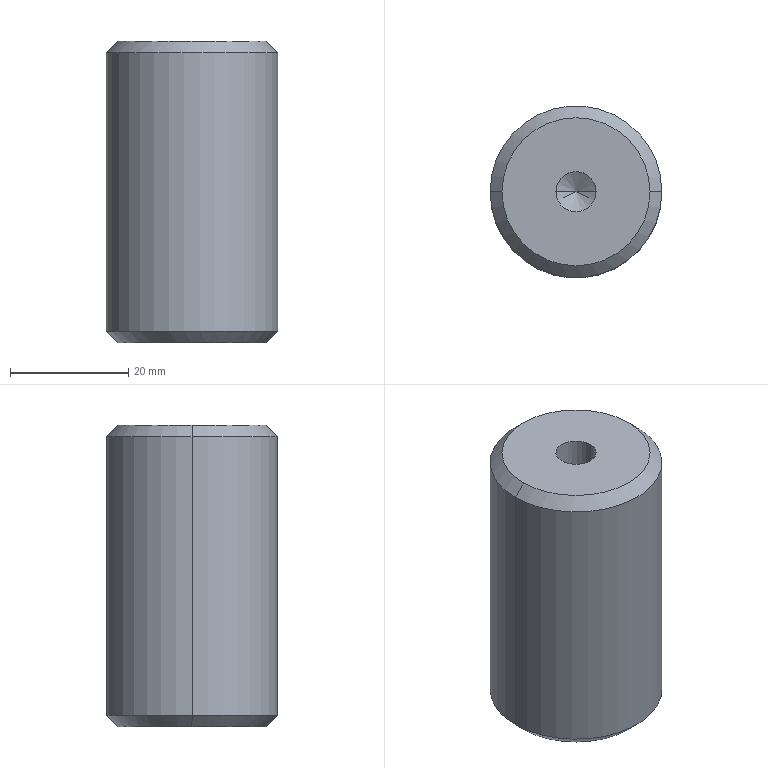Part | STEP file | BU-A03b#180 | 1 solid | 16 faces | box 29 x 29 x 51 mm | volume 31619 mm3 | cone 8 | cylinder 6 | plane 2 | commonest cylinder face diameters 6.8 x4 29 x2
STEP:
#1=CARTESIAN_POINT('',(0.,0.,0.));
#2=DIRECTION('',(0.,0.,1.));
#3=DIRECTION('',(1.,0.,0.));
#4=AXIS2_PLACEMENT_3D('',#1,#2,#3);
#5=CARTESIAN_POINT('',(12.5,0.,51.));
#6=VERTEX_POINT('',#5);
#7=CARTESIAN_POINT('',(-12.5,0.,51.));
#8=VERTEX_POINT('',#7);
#9=CARTESIAN_POINT('',(0.,0.,51.));
#10=DIRECTION('',(0.,0.,1.));
#11=DIRECTION('',(1.,0.,0.));
#12=AXIS2_PLACEMENT_3D('',#9,#10,#11);
#13=CIRCLE('',#12,12.5);
#14=CARTESIAN_POINT('',(0.,0.,51.));
#15=DIRECTION('',(0.,0.,-1.));
#16=DIRECTION('',(-1.,0.,0.));
#17=AXIS2_PLACEMENT_3D('',#14,#15,#16);
#18=CONICAL_SURFACE('',#17,12.5,0.7854);
#19=CARTESIAN_POINT('',(3.142,0.));
#20=DIRECTION('',(-1.,0.));
#21=VECTOR('',#20,1.);
#22=LINE('',#19,#21);
#23=(GEOMETRIC_REPRESENTATION_CONTEXT(2)PARAMETRIC_REPRESENTATION_CONTEXT()REPRESENTATION_CONTEXT('',''));
#24=DEFINITIONAL_REPRESENTATION('',(#22),#23);
#25=PCURVE('',#18,#24);
#26=CARTESIAN_POINT('',(0.,0.,51.));
#27=DIRECTION('',(0.,0.,1.));
#28=DIRECTION('',(1.,0.,0.));
#29=AXIS2_PLACEMENT_3D('',#26,#27,#28);
#30=PLANE('',#29);
#31=CARTESIAN_POINT('',(0.,0.));
#32=DIRECTION('',(1.,0.));
#33=AXIS2_PLACEMENT_2D('',#31,#32);
#34=CIRCLE('',#33,12.5);
#35=(GEOMETRIC_REPRESENTATION_CONTEXT(2)PARAMETRIC_REPRESENTATION_CONTEXT()REPRESENTATION_CONTEXT('',''));
#36=DEFINITIONAL_REPRESENTATION('',(#34),#35);
#37=PCURVE('',#30,#36);
#38=SURFACE_CURVE('',#13,(#25,#37),.PCURVE_S1.);
#39=EDGE_CURVE('',#6,#8,#38,.T.);
#40=ORIENTED_EDGE('',*,*,#39,.F.);
#41=CARTESIAN_POINT('',(14.5,0.,49.));
#42=VERTEX_POINT('',#41);
#43=CARTESIAN_POINT('',(12.5,0.,51.));
#44=DIRECTION('',(0.7071,0.,-0.7071));
#45=VECTOR('',#44,1.);
#46=LINE('',#43,#45);
#47=CARTESIAN_POINT('',(3.142,0.));
#48=DIRECTION('',(0.,1.));
#49=VECTOR('',#48,1.);
#50=LINE('',#47,#49);
#51=(GEOMETRIC_REPRESENTATION_CONTEXT(2)PARAMETRIC_REPRESENTATION_CONTEXT()REPRESENTATION_CONTEXT('',''));
#52=DEFINITIONAL_REPRESENTATION('',(#50),#51);
#53=PCURVE('',#18,#52);
#54=CARTESIAN_POINT('',(0.,0.,51.));
#55=DIRECTION('',(0.,0.,-1.));
#56=DIRECTION('',(-1.,0.,0.));
#57=AXIS2_PLACEMENT_3D('',#54,#55,#56);
#58=CONICAL_SURFACE('',#57,12.5,0.7854);
#59=CARTESIAN_POINT('',(3.142,0.));
#60=DIRECTION('',(0.,1.));
#61=VECTOR('',#60,1.);
#62=LINE('',#59,#61);
#63=(GEOMETRIC_REPRESENTATION_CONTEXT(2)PARAMETRIC_REPRESENTATION_CONTEXT()REPRESENTATION_CONTEXT('',''));
#64=DEFINITIONAL_REPRESENTATION('',(#62),#63);
#65=PCURVE('',#58,#64);
#66=SURFACE_CURVE('',#46,(#53,#65),.PCURVE_S1.);
#67=EDGE_CURVE('',#6,#42,#66,.T.);
#68=ORIENTED_EDGE('',*,*,#67,.T.);
#69=CARTESIAN_POINT('',(-14.5,0.,49.));
#70=VERTEX_POINT('',#69);
#71=CARTESIAN_POINT('',(0.,0.,49.));
#72=DIRECTION('',(0.,0.,-1.));
#73=DIRECTION('',(1.,0.,0.));
#74=AXIS2_PLACEMENT_3D('',#71,#72,#73);
#75=CIRCLE('',#74,14.5);
#76=CARTESIAN_POINT('',(-3.142,2.));
#77=DIRECTION('',(1.,0.));
#78=VECTOR('',#77,1.);
#79=LINE('',#76,#78);
#80=(GEOMETRIC_REPRESENTATION_CONTEXT(2)PARAMETRIC_REPRESENTATION_CONTEXT()REPRESENTATION_CONTEXT('',''));
#81=DEFINITIONAL_REPRESENTATION('',(#79),#80);
#82=PCURVE('',#18,#81);
#83=CARTESIAN_POINT('',(0.,0.,51.));
#84=DIRECTION('',(0.,0.,-1.));
#85=DIRECTION('',(-1.,0.,0.));
#86=AXIS2_PLACEMENT_3D('',#83,#84,#85);
#87=CYLINDRICAL_SURFACE('',#86,14.5);
#88=CARTESIAN_POINT('',(-3.142,2.));
#89=DIRECTION('',(1.,0.));
#90=VECTOR('',#89,1.);
#91=LINE('',#88,#90);
#92=(GEOMETRIC_REPRESENTATION_CONTEXT(2)PARAMETRIC_REPRESENTATION_CONTEXT()REPRESENTATION_CONTEXT('',''));
#93=DEFINITIONAL_REPRESENTATION('',(#91),#92);
#94=PCURVE('',#87,#93);
#95=SURFACE_CURVE('',#75,(#82,#94),.PCURVE_S1.);
#96=EDGE_CURVE('',#70,#42,#95,.T.);
#97=ORIENTED_EDGE('',*,*,#96,.F.);
#98=CARTESIAN_POINT('',(-12.5,0.,51.));
#99=DIRECTION('',(-0.7071,0.,-0.7071));
#100=VECTOR('',#99,1.);
#101=LINE('',#98,#100);
#102=CARTESIAN_POINT('',(0.,0.));
#103=DIRECTION('',(0.,1.));
#104=VECTOR('',#103,1.);
#105=LINE('',#102,#104);
#106=(GEOMETRIC_REPRESENTATION_CONTEXT(2)PARAMETRIC_REPRESENTATION_CONTEXT()REPRESENTATION_CONTEXT('',''));
#107=DEFINITIONAL_REPRESENTATION('',(#105),#106);
#108=PCURVE('',#18,#107);
#109=CARTESIAN_POINT('',(6.283,0.));
#110=DIRECTION('',(0.,1.));
#111=VECTOR('',#110,1.);
#112=LINE('',#109,#111);
#113=(GEOMETRIC_REPRESENTATION_CONTEXT(2)PARAMETRIC_REPRESENTATION_CONTEXT()REPRESENTATION_CONTEXT('',''));
#114=DEFINITIONAL_REPRESENTATION('',(#112),#113);
#115=PCURVE('',#58,#114);
#116=SURFACE_CURVE('',#101,(#108,#115),.PCURVE_S1.);
#117=EDGE_CURVE('',#8,#70,#116,.T.);
#118=ORIENTED_EDGE('',*,*,#117,.F.);
#119=EDGE_LOOP('',(#40,#68,#97,#118));
#120=FACE_BOUND('',#119,.T.);
#121=ADVANCED_FACE('',(#120),#18,.T.);
#122=CARTESIAN_POINT('',(-12.5,0.,0.));
#123=VERTEX_POINT('',#122);
#124=CARTESIAN_POINT('',(12.5,0.,0.));
#125=VERTEX_POINT('',#124);
#126=CARTESIAN_POINT('',(0.,0.,0.));
#127=DIRECTION('',(0.,0.,-1.));
#128=DIRECTION('',(1.,0.,0.));
#129=AXIS2_PLACEMENT_3D('',#126,#127,#128);
#130=CIRCLE('',#129,12.5);
#131=CARTESIAN_POINT('',(0.,0.,2.));
#132=DIRECTION('',(0.,0.,1.));
#133=DIRECTION('',(1.,0.,0.));
#134=AXIS2_PLACEMENT_3D('',#131,#132,#133);
#135=CONICAL_SURFACE('',#134,14.5,0.7854);
#136=CARTESIAN_POINT('',(6.283,-2.));
#137=DIRECTION('',(-1.,0.));
#138=VECTOR('',#137,1.);
#139=LINE('',#136,#138);
#140=(GEOMETRIC_REPRESENTATION_CONTEXT(2)PARAMETRIC_REPRESENTATION_CONTEXT()REPRESENTATION_CONTEXT('',''));
#141=DEFINITIONAL_REPRESENTATION('',(#139),#140);
#142=PCURVE('',#135,#141);
#143=CARTESIAN_POINT('',(0.,0.,0.));
#144=DIRECTION('',(0.,0.,1.));
#145=DIRECTION('',(1.,0.,0.));
#146=AXIS2_PLACEMENT_3D('',#143,#144,#145);
#147=PLANE('',#146);
#148=CARTESIAN_POINT('',(12.5,0.));
#149=CARTESIAN_POINT('',(12.5,-21.651));
#150=CARTESIAN_POINT('',(-6.25,-10.825));
#151=CARTESIAN_POINT('',(-25.,0.));
#152=CARTESIAN_POINT('',(-6.25,10.825));
#153=CARTESIAN_POINT('',(12.5,21.651));
#154=CARTESIAN_POINT('',(12.5,0.));
#155=(BOUNDED_CURVE()B_SPLINE_CURVE(2,(#148,#149,#150,#151,#152,#153,#154),.UNSPECIFIED.,.T.,.F.)B_SPLINE_CURVE_WITH_KNOTS((1,2,2,2,2,1),(-2.094,0.,2.094,4.189,6.283,8.378),.UNSPECIFIED.)CURVE()GEOMETRIC_REPRESENTATION_ITEM()RATIONAL_B_SPLINE_CURVE((1.,0.5,1.,0.5,1.,0.5,1.))REPRESENTATION_ITEM(''));
#156=(GEOMETRIC_REPRESENTATION_CONTEXT(2)PARAMETRIC_REPRESENTATION_CONTEXT()REPRESENTATION_CONTEXT('',''));
#157=DEFINITIONAL_REPRESENTATION('',(#155),#156);
#158=PCURVE('',#147,#157);
#159=SURFACE_CURVE('',#130,(#142,#158),.PCURVE_S1.);
#160=EDGE_CURVE('',#123,#125,#159,.T.);
#161=ORIENTED_EDGE('',*,*,#160,.F.);
#162=CARTESIAN_POINT('',(-14.5,0.,2.));
#163=VERTEX_POINT('',#162);
#164=CARTESIAN_POINT('',(-14.5,0.,2.));
#165=DIRECTION('',(-0.7071,0.,0.7071));
#166=VECTOR('',#165,1.);
#167=LINE('',#164,#166);
#168=CARTESIAN_POINT('',(3.142,0.));
#169=DIRECTION('',(0.,1.));
#170=VECTOR('',#169,1.);
#171=LINE('',#168,#170);
#172=(GEOMETRIC_REPRESENTATION_CONTEXT(2)PARAMETRIC_REPRESENTATION_CONTEXT()REPRESENTATION_CONTEXT('',''));
#173=DEFINITIONAL_REPRESENTATION('',(#171),#172);
#174=PCURVE('',#135,#173);
#175=CARTESIAN_POINT('',(0.,0.,2.));
#176=DIRECTION('',(0.,0.,1.));
#177=DIRECTION('',(1.,0.,0.));
#178=AXIS2_PLACEMENT_3D('',#175,#176,#177);
#179=CONICAL_SURFACE('',#178,14.5,0.7854);
#180=CARTESIAN_POINT('',(3.142,0.));
#181=DIRECTION('',(0.,1.));
#182=VECTOR('',#181,1.);
#183=LINE('',#180,#182);
#184=(GEOMETRIC_REPRESENTATION_CONTEXT(2)PARAMETRIC_REPRESENTATION_CONTEXT()REPRESENTATION_CONTEXT('',''));
#185=DEFINITIONAL_REPRESENTATION('',(#183),#184);
#186=PCURVE('',#179,#185);
#187=SURFACE_CURVE('',#167,(#174,#186),.PCURVE_S1.);
#188=EDGE_CURVE('',#123,#163,#187,.T.);
#189=ORIENTED_EDGE('',*,*,#188,.T.);
#190=CARTESIAN_POINT('',(14.5,0.,2.));
#191=VERTEX_POINT('',#190);
#192=CARTESIAN_POINT('',(0.,0.,2.));
#193=DIRECTION('',(0.,0.,1.));
#194=DIRECTION('',(1.,0.,0.));
#195=AXIS2_PLACEMENT_3D('',#192,#193,#194);
#196=CIRCLE('',#195,14.5);
#197=CARTESIAN_POINT('',(0.,0.));
#198=DIRECTION('',(1.,0.));
#199=VECTOR('',#198,1.);
#200=LINE('',#197,#199);
#201=(GEOMETRIC_REPRESENTATION_CONTEXT(2)PARAMETRIC_REPRESENTATION_CONTEXT()REPRESENTATION_CONTEXT('',''));
#202=DEFINITIONAL_REPRESENTATION('',(#200),#201);
#203=PCURVE('',#135,#202);
#204=CARTESIAN_POINT('',(3.142,49.));
#205=DIRECTION('',(-1.,0.));
#206=VECTOR('',#205,1.);
#207=LINE('',#204,#206);
#208=(GEOMETRIC_REPRESENTATION_CONTEXT(2)PARAMETRIC_REPRESENTATION_CONTEXT()REPRESENTATION_CONTEXT('',''));
#209=DEFINITIONAL_REPRESENTATION('',(#207),#208);
#210=PCURVE('',#87,#209);
#211=SURFACE_CURVE('',#196,(#203,#210),.PCURVE_S1.);
#212=EDGE_CURVE('',#191,#163,#211,.T.);
#213=ORIENTED_EDGE('',*,*,#212,.F.);
#214=CARTESIAN_POINT('',(14.5,0.,2.));
#215=DIRECTION('',(0.7071,0.,0.7071));
#216=VECTOR('',#215,1.);
#217=LINE('',#214,#216);
#218=CARTESIAN_POINT('',(0.,0.));
#219=DIRECTION('',(0.,1.));
#220=VECTOR('',#219,1.);
#221=LINE('',#218,#220);
#222=(GEOMETRIC_REPRESENTATION_CONTEXT(2)PARAMETRIC_REPRESENTATION_CONTEXT()REPRESENTATION_CONTEXT('',''));
#223=DEFINITIONAL_REPRESENTATION('',(#221),#222);
#224=PCURVE('',#135,#223);
#225=CARTESIAN_POINT('',(6.283,0.));
#226=DIRECTION('',(0.,1.));
#227=VECTOR('',#226,1.);
#228=LINE('',#225,#227);
#229=(GEOMETRIC_REPRESENTATION_CONTEXT(2)PARAMETRIC_REPRESENTATION_CONTEXT()REPRESENTATION_CONTEXT('',''));
#230=DEFINITIONAL_REPRESENTATION('',(#228),#229);
#231=PCURVE('',#179,#230);
#232=SURFACE_CURVE('',#217,(#224,#231),.PCURVE_S1.);
#233=EDGE_CURVE('',#125,#191,#232,.T.);
#234=ORIENTED_EDGE('',*,*,#233,.F.);
#235=EDGE_LOOP('',(#161,#189,#213,#234));
#236=FACE_BOUND('',#235,.T.);
#237=ADVANCED_FACE('',(#236),#135,.T.);
#238=CARTESIAN_POINT('',(-3.4,0.,28.));
#239=VERTEX_POINT('',#238);
#240=CARTESIAN_POINT('',(3.4,0.,28.));
#241=VERTEX_POINT('',#240);
#242=CARTESIAN_POINT('',(0.,0.,28.));
#243=DIRECTION('',(0.,0.,1.));
#244=DIRECTION('',(1.,0.,0.));
#245=AXIS2_PLACEMENT_3D('',#242,#243,#244);
#246=CIRCLE('',#245,3.4);
#247=CARTESIAN_POINT('',(0.,0.,28.));
#248=DIRECTION('',(0.,0.,1.));
#249=DIRECTION('',(1.,0.,0.));
#250=AXIS2_PLACEMENT_3D('',#247,#248,#249);
#251=CONICAL_SURFACE('',#250,3.4,1.03);
#252=CARTESIAN_POINT('',(0.,0.));
#253=DIRECTION('',(1.,0.));
#254=VECTOR('',#253,1.);
#255=LINE('',#252,#254);
#256=(GEOMETRIC_REPRESENTATION_CONTEXT(2)PARAMETRIC_REPRESENTATION_CONTEXT()REPRESENTATION_CONTEXT('',''));
#257=DEFINITIONAL_REPRESENTATION('',(#255),#256);
#258=PCURVE('',#251,#257);
#259=CARTESIAN_POINT('',(0.,0.,51.));
#260=DIRECTION('',(0.,0.,1.));
#261=DIRECTION('',(1.,0.,0.));
#262=AXIS2_PLACEMENT_3D('',#259,#260,#261);
#263=CYLINDRICAL_SURFACE('',#262,3.4);
#264=CARTESIAN_POINT('',(0.,-23.));
#265=DIRECTION('',(1.,0.));
#266=VECTOR('',#265,1.);
#267=LINE('',#264,#266);
#268=(GEOMETRIC_REPRESENTATION_CONTEXT(2)PARAMETRIC_REPRESENTATION_CONTEXT()REPRESENTATION_CONTEXT('',''));
#269=DEFINITIONAL_REPRESENTATION('',(#267),#268);
#270=PCURVE('',#263,#269);
#271=SURFACE_CURVE('',#246,(#258,#270),.PCURVE_S1.);
#272=EDGE_CURVE('',#239,#241,#271,.T.);
#273=ORIENTED_EDGE('',*,*,#272,.F.);
#274=CARTESIAN_POINT('',(0.,0.,25.957));
#275=VERTEX_POINT('',#274);
#276=CARTESIAN_POINT('',(-3.4,0.,28.));
#277=DIRECTION('',(-0.8572,0.,0.515));
#278=VECTOR('',#277,1.);
#279=LINE('',#276,#278);
#280=CARTESIAN_POINT('',(3.142,0.));
#281=DIRECTION('',(0.,1.));
#282=VECTOR('',#281,1.);
#283=LINE('',#280,#282);
#284=(GEOMETRIC_REPRESENTATION_CONTEXT(2)PARAMETRIC_REPRESENTATION_CONTEXT()REPRESENTATION_CONTEXT('',''));
#285=DEFINITIONAL_REPRESENTATION('',(#283),#284);
#286=PCURVE('',#251,#285);
#287=CARTESIAN_POINT('',(0.,0.,28.));
#288=DIRECTION('',(0.,0.,1.));
#289=DIRECTION('',(1.,0.,0.));
#290=AXIS2_PLACEMENT_3D('',#287,#288,#289);
#291=CONICAL_SURFACE('',#290,3.4,1.03);
#292=CARTESIAN_POINT('',(3.142,0.));
#293=DIRECTION('',(0.,1.));
#294=VECTOR('',#293,1.);
#295=LINE('',#292,#294);
#296=(GEOMETRIC_REPRESENTATION_CONTEXT(2)PARAMETRIC_REPRESENTATION_CONTEXT()REPRESENTATION_CONTEXT('',''));
#297=DEFINITIONAL_REPRESENTATION('',(#295),#296);
#298=PCURVE('',#291,#297);
#299=SURFACE_CURVE('',#279,(#286,#298),.PCURVE_S1.);
#300=EDGE_CURVE('',#275,#239,#299,.T.);
#301=ORIENTED_EDGE('',*,*,#300,.F.);
#302=CARTESIAN_POINT('',(3.4,0.,28.));
#303=DIRECTION('',(0.8572,0.,0.515));
#304=VECTOR('',#303,1.);
#305=LINE('',#302,#304);
#306=CARTESIAN_POINT('',(6.283,-2.043));
#307=CARTESIAN_POINT('',(6.283,-2.012));
#308=CARTESIAN_POINT('',(6.283,-1.95));
#309=CARTESIAN_POINT('',(6.283,-1.857));
#310=CARTESIAN_POINT('',(6.283,-1.764));
#311=CARTESIAN_POINT('',(6.283,-1.671));
#312=CARTESIAN_POINT('',(6.283,-1.579));
#313=CARTESIAN_POINT('',(6.283,-1.486));
#314=CARTESIAN_POINT('',(6.283,-1.393));
#315=CARTESIAN_POINT('',(6.283,-1.3));
#316=CARTESIAN_POINT('',(6.283,-1.207));
#317=CARTESIAN_POINT('',(6.283,-1.114));
#318=CARTESIAN_POINT('',(6.283,-1.021));
#319=CARTESIAN_POINT('',(6.283,-0.9286));
#320=CARTESIAN_POINT('',(6.283,-0.8357));
#321=CARTESIAN_POINT('',(6.283,-0.7429));
#322=CARTESIAN_POINT('',(6.283,-0.65));
#323=CARTESIAN_POINT('',(6.283,-0.5572));
#324=CARTESIAN_POINT('',(6.283,-0.4643));
#325=CARTESIAN_POINT('',(6.283,-0.3714));
#326=CARTESIAN_POINT('',(6.283,-0.2786));
#327=CARTESIAN_POINT('',(6.283,-0.1857));
#328=CARTESIAN_POINT('',(6.283,-0.09286));
#329=CARTESIAN_POINT('',(6.283,-0.03095));
#330=CARTESIAN_POINT('',(6.283,0.));
#331=B_SPLINE_CURVE_WITH_KNOTS('',3,(#306,#307,#308,#309,#310,#311,#312,#313,#314,#315,#316,#317,#318,#319,#320,#321,#322,#323,#324,#325,#326,#327,#328,#329,#330),.UNSPECIFIED.,.F.,.F.,(4,1,1,1,1,1,1,1,1,1,1,1,1,1,1,1,1,1,1,1,1,1,4),(-3.967,-3.786,-3.606,-3.426,-3.245,-3.065,-2.885,-2.704,-2.524,-2.344,-2.164,-1.983,-1.803,-1.623,-1.442,-1.262,-1.082,-0.9015,-0.7212,-0.5409,-0.3606,-0.1803,0.),.QUASI_UNIFORM_KNOTS.);
#332=(GEOMETRIC_REPRESENTATION_CONTEXT(2)PARAMETRIC_REPRESENTATION_CONTEXT()REPRESENTATION_CONTEXT('',''));
#333=DEFINITIONAL_REPRESENTATION('',(#331),#332);
#334=PCURVE('',#251,#333);
#335=CARTESIAN_POINT('',(0.,-2.043));
#336=CARTESIAN_POINT('',(0.,-2.012));
#337=CARTESIAN_POINT('',(0.,-1.95));
#338=CARTESIAN_POINT('',(0.,-1.857));
#339=CARTESIAN_POINT('',(0.,-1.764));
#340=CARTESIAN_POINT('',(0.,-1.671));
#341=CARTESIAN_POINT('',(0.,-1.579));
#342=CARTESIAN_POINT('',(0.,-1.486));
#343=CARTESIAN_POINT('',(0.,-1.393));
#344=CARTESIAN_POINT('',(0.,-1.3));
#345=CARTESIAN_POINT('',(0.,-1.207));
#346=CARTESIAN_POINT('',(0.,-1.114));
#347=CARTESIAN_POINT('',(0.,-1.021));
#348=CARTESIAN_POINT('',(0.,-0.9286));
#349=CARTESIAN_POINT('',(0.,-0.8357));
#350=CARTESIAN_POINT('',(0.,-0.7429));
#351=CARTESIAN_POINT('',(0.,-0.65));
#352=CARTESIAN_POINT('',(0.,-0.5572));
#353=CARTESIAN_POINT('',(0.,-0.4643));
#354=CARTESIAN_POINT('',(0.,-0.3714));
#355=CARTESIAN_POINT('',(0.,-0.2786));
#356=CARTESIAN_POINT('',(0.,-0.1857));
#357=CARTESIAN_POINT('',(0.,-0.09286));
#358=CARTESIAN_POINT('',(0.,-0.03095));
#359=CARTESIAN_POINT('',(0.,0.));
#360=B_SPLINE_CURVE_WITH_KNOTS('',3,(#335,#336,#337,#338,#339,#340,#341,#342,#343,#344,#345,#346,#347,#348,#349,#350,#351,#352,#353,#354,#355,#356,#357,#358,#359),.UNSPECIFIED.,.F.,.F.,(4,1,1,1,1,1,1,1,1,1,1,1,1,1,1,1,1,1,1,1,1,1,4),(-3.967,-3.786,-3.606,-3.426,-3.245,-3.065,-2.885,-2.704,-2.524,-2.344,-2.164,-1.983,-1.803,-1.623,-1.442,-1.262,-1.082,-0.9015,-0.7212,-0.5409,-0.3606,-0.1803,0.),.QUASI_UNIFORM_KNOTS.);
#361=(GEOMETRIC_REPRESENTATION_CONTEXT(2)PARAMETRIC_REPRESENTATION_CONTEXT()REPRESENTATION_CONTEXT('',''));
#362=DEFINITIONAL_REPRESENTATION('',(#360),#361);
#363=PCURVE('',#291,#362);
#364=SURFACE_CURVE('',#305,(#334,#363),.PCURVE_S1.);
#365=EDGE_CURVE('',#275,#241,#364,.T.);
#366=ORIENTED_EDGE('',*,*,#365,.T.);
#367=EDGE_LOOP('',(#273,#301,#366));
#368=FACE_BOUND('',#367,.F.);
#369=ADVANCED_FACE('',(#368),#251,.F.);
#370=CARTESIAN_POINT('',(3.4,0.,51.));
#371=VERTEX_POINT('',#370);
#372=CARTESIAN_POINT('',(3.4,0.,51.));
#373=DIRECTION('',(0.,0.,1.));
#374=VECTOR('',#373,1.);
#375=LINE('',#372,#374);
#376=CARTESIAN_POINT('',(6.283,0.));
#377=DIRECTION('',(0.,1.));
#378=VECTOR('',#377,1.);
#379=LINE('',#376,#378);
#380=(GEOMETRIC_REPRESENTATION_CONTEXT(2)PARAMETRIC_REPRESENTATION_CONTEXT()REPRESENTATION_CONTEXT('',''));
#381=DEFINITIONAL_REPRESENTATION('',(#379),#380);
#382=PCURVE('',#263,#381);
#383=CARTESIAN_POINT('',(0.,0.,51.));
#384=DIRECTION('',(0.,0.,1.));
#385=DIRECTION('',(1.,0.,0.));
#386=AXIS2_PLACEMENT_3D('',#383,#384,#385);
#387=CYLINDRICAL_SURFACE('',#386,3.4);
#388=CARTESIAN_POINT('',(0.,0.));
#389=DIRECTION('',(0.,1.));
#390=VECTOR('',#389,1.);
#391=LINE('',#388,#390);
#392=(GEOMETRIC_REPRESENTATION_CONTEXT(2)PARAMETRIC_REPRESENTATION_CONTEXT()REPRESENTATION_CONTEXT('',''));
#393=DEFINITIONAL_REPRESENTATION('',(#391),#392);
#394=PCURVE('',#387,#393);
#395=SURFACE_CURVE('',#375,(#382,#394),.PCURVE_S1.);
#396=EDGE_CURVE('',#241,#371,#395,.T.);
#397=ORIENTED_EDGE('',*,*,#396,.T.);
#398=CARTESIAN_POINT('',(-3.4,0.,51.));
#399=VERTEX_POINT('',#398);
#400=CARTESIAN_POINT('',(0.,0.,51.));
#401=DIRECTION('',(0.,0.,1.));
#402=DIRECTION('',(1.,0.,0.));
#403=AXIS2_PLACEMENT_3D('',#400,#401,#402);
#404=CIRCLE('',#403,3.4);
#405=CARTESIAN_POINT('',(0.,0.));
#406=DIRECTION('',(1.,0.));
#407=VECTOR('',#406,1.);
#408=LINE('',#405,#407);
#409=(GEOMETRIC_REPRESENTATION_CONTEXT(2)PARAMETRIC_REPRESENTATION_CONTEXT()REPRESENTATION_CONTEXT('',''));
#410=DEFINITIONAL_REPRESENTATION('',(#408),#409);
#411=PCURVE('',#263,#410);
#412=CARTESIAN_POINT('',(0.,0.));
#413=DIRECTION('',(1.,0.));
#414=AXIS2_PLACEMENT_2D('',#412,#413);
#415=CIRCLE('',#414,3.4);
#416=(GEOMETRIC_REPRESENTATION_CONTEXT(2)PARAMETRIC_REPRESENTATION_CONTEXT()REPRESENTATION_CONTEXT('',''));
#417=DEFINITIONAL_REPRESENTATION('',(#415),#416);
#418=PCURVE('',#30,#417);
#419=SURFACE_CURVE('',#404,(#411,#418),.PCURVE_S1.);
#420=EDGE_CURVE('',#399,#371,#419,.T.);
#421=ORIENTED_EDGE('',*,*,#420,.F.);
#422=CARTESIAN_POINT('',(-3.4,0.,51.));
#423=DIRECTION('',(0.,0.,1.));
#424=VECTOR('',#423,1.);
#425=LINE('',#422,#424);
#426=CARTESIAN_POINT('',(3.142,0.));
#427=DIRECTION('',(0.,1.));
#428=VECTOR('',#427,1.);
#429=LINE('',#426,#428);
#430=(GEOMETRIC_REPRESENTATION_CONTEXT(2)PARAMETRIC_REPRESENTATION_CONTEXT()REPRESENTATION_CONTEXT('',''));
#431=DEFINITIONAL_REPRESENTATION('',(#429),#430);
#432=PCURVE('',#263,#431);
#433=CARTESIAN_POINT('',(3.142,0.));
#434=DIRECTION('',(0.,1.));
#435=VECTOR('',#434,1.);
#436=LINE('',#433,#435);
#437=(GEOMETRIC_REPRESENTATION_CONTEXT(2)PARAMETRIC_REPRESENTATION_CONTEXT()REPRESENTATION_CONTEXT('',''));
#438=DEFINITIONAL_REPRESENTATION('',(#436),#437);
#439=PCURVE('',#387,#438);
#440=SURFACE_CURVE('',#425,(#432,#439),.PCURVE_S1.);
#441=EDGE_CURVE('',#239,#399,#440,.T.);
#442=ORIENTED_EDGE('',*,*,#441,.F.);
#443=ORIENTED_EDGE('',*,*,#272,.T.);
#444=EDGE_LOOP('',(#397,#421,#442,#443));
#445=FACE_BOUND('',#444,.F.);
#446=ADVANCED_FACE('',(#445),#263,.F.);
#447=CARTESIAN_POINT('',(3.4,0.,23.));
#448=VERTEX_POINT('',#447);
#449=CARTESIAN_POINT('',(-3.4,0.,23.));
#450=VERTEX_POINT('',#449);
#451=CARTESIAN_POINT('',(0.,0.,23.));
#452=DIRECTION('',(0.,0.,-1.));
#453=DIRECTION('',(-1.,0.,0.));
#454=AXIS2_PLACEMENT_3D('',#451,#452,#453);
#455=CIRCLE('',#454,3.4);
#456=CARTESIAN_POINT('',(0.,0.,23.));
#457=DIRECTION('',(0.,0.,-1.));
#458=DIRECTION('',(-1.,0.,0.));
#459=AXIS2_PLACEMENT_3D('',#456,#457,#458);
#460=CONICAL_SURFACE('',#459,3.4,1.03);
#461=CARTESIAN_POINT('',(0.,0.));
#462=DIRECTION('',(1.,0.));
#463=VECTOR('',#462,1.);
#464=LINE('',#461,#463);
#465=(GEOMETRIC_REPRESENTATION_CONTEXT(2)PARAMETRIC_REPRESENTATION_CONTEXT()REPRESENTATION_CONTEXT('',''));
#466=DEFINITIONAL_REPRESENTATION('',(#464),#465);
#467=PCURVE('',#460,#466);
#468=CARTESIAN_POINT('',(0.,0.,0.));
#469=DIRECTION('',(0.,0.,-1.));
#470=DIRECTION('',(-1.,0.,0.));
#471=AXIS2_PLACEMENT_3D('',#468,#469,#470);
#472=CYLINDRICAL_SURFACE('',#471,3.4);
#473=CARTESIAN_POINT('',(0.,-23.));
#474=DIRECTION('',(1.,0.));
#475=VECTOR('',#474,1.);
#476=LINE('',#473,#475);
#477=(GEOMETRIC_REPRESENTATION_CONTEXT(2)PARAMETRIC_REPRESENTATION_CONTEXT()REPRESENTATION_CONTEXT('',''));
#478=DEFINITIONAL_REPRESENTATION('',(#476),#477);
#479=PCURVE('',#472,#478);
#480=SURFACE_CURVE('',#455,(#467,#479),.PCURVE_S1.);
#481=EDGE_CURVE('',#448,#450,#480,.T.);
#482=ORIENTED_EDGE('',*,*,#481,.F.);
#483=CARTESIAN_POINT('',(0.,0.,25.043));
#484=VERTEX_POINT('',#483);
#485=CARTESIAN_POINT('',(3.4,0.,23.));
#486=DIRECTION('',(0.8572,0.,-0.515));
#487=VECTOR('',#486,1.);
#488=LINE('',#485,#487);
#489=CARTESIAN_POINT('',(3.142,0.));
#490=DIRECTION('',(0.,1.));
#491=VECTOR('',#490,1.);
#492=LINE('',#489,#491);
#493=(GEOMETRIC_REPRESENTATION_CONTEXT(2)PARAMETRIC_REPRESENTATION_CONTEXT()REPRESENTATION_CONTEXT('',''));
#494=DEFINITIONAL_REPRESENTATION('',(#492),#493);
#495=PCURVE('',#460,#494);
#496=CARTESIAN_POINT('',(0.,0.,23.));
#497=DIRECTION('',(0.,0.,-1.));
#498=DIRECTION('',(-1.,0.,0.));
#499=AXIS2_PLACEMENT_3D('',#496,#497,#498);
#500=CONICAL_SURFACE('',#499,3.4,1.03);
#501=CARTESIAN_POINT('',(3.142,0.));
#502=DIRECTION('',(0.,1.));
#503=VECTOR('',#502,1.);
#504=LINE('',#501,#503);
#505=(GEOMETRIC_REPRESENTATION_CONTEXT(2)PARAMETRIC_REPRESENTATION_CONTEXT()REPRESENTATION_CONTEXT('',''));
#506=DEFINITIONAL_REPRESENTATION('',(#504),#505);
#507=PCURVE('',#500,#506);
#508=SURFACE_CURVE('',#488,(#495,#507),.PCURVE_S1.);
#509=EDGE_CURVE('',#484,#448,#508,.T.);
#510=ORIENTED_EDGE('',*,*,#509,.F.);
#511=CARTESIAN_POINT('',(-3.4,0.,23.));
#512=DIRECTION('',(-0.8572,0.,-0.515));
#513=VECTOR('',#512,1.);
#514=LINE('',#511,#513);
#515=CARTESIAN_POINT('',(6.283,0.));
#516=DIRECTION('',(0.,1.));
#517=VECTOR('',#516,1.);
#518=LINE('',#515,#517);
#519=(GEOMETRIC_REPRESENTATION_CONTEXT(2)PARAMETRIC_REPRESENTATION_CONTEXT()REPRESENTATION_CONTEXT('',''));
#520=DEFINITIONAL_REPRESENTATION('',(#518),#519);
#521=PCURVE('',#460,#520);
#522=CARTESIAN_POINT('',(0.,0.));
#523=DIRECTION('',(0.,1.));
#524=VECTOR('',#523,1.);
#525=LINE('',#522,#524);
#526=(GEOMETRIC_REPRESENTATION_CONTEXT(2)PARAMETRIC_REPRESENTATION_CONTEXT()REPRESENTATION_CONTEXT('',''));
#527=DEFINITIONAL_REPRESENTATION('',(#525),#526);
#528=PCURVE('',#500,#527);
#529=SURFACE_CURVE('',#514,(#521,#528),.PCURVE_S1.);
#530=EDGE_CURVE('',#484,#450,#529,.T.);
#531=ORIENTED_EDGE('',*,*,#530,.T.);
#532=EDGE_LOOP('',(#482,#510,#531));
#533=FACE_BOUND('',#532,.F.);
#534=ADVANCED_FACE('',(#533),#460,.F.);
#535=CARTESIAN_POINT('',(-3.4,0.,0.));
#536=VERTEX_POINT('',#535);
#537=CARTESIAN_POINT('',(-3.4,0.,0.));
#538=DIRECTION('',(0.,0.,-1.));
#539=VECTOR('',#538,1.);
#540=LINE('',#537,#539);
#541=CARTESIAN_POINT('',(6.283,0.));
#542=DIRECTION('',(0.,1.));
#543=VECTOR('',#542,1.);
#544=LINE('',#541,#543);
#545=(GEOMETRIC_REPRESENTATION_CONTEXT(2)PARAMETRIC_REPRESENTATION_CONTEXT()REPRESENTATION_CONTEXT('',''));
#546=DEFINITIONAL_REPRESENTATION('',(#544),#545);
#547=PCURVE('',#472,#546);
#548=CARTESIAN_POINT('',(0.,0.,0.));
#549=DIRECTION('',(0.,0.,-1.));
#550=DIRECTION('',(-1.,0.,0.));
#551=AXIS2_PLACEMENT_3D('',#548,#549,#550);
#552=CYLINDRICAL_SURFACE('',#551,3.4);
#553=CARTESIAN_POINT('',(0.,0.));
#554=DIRECTION('',(0.,1.));
#555=VECTOR('',#554,1.);
#556=LINE('',#553,#555);
#557=(GEOMETRIC_REPRESENTATION_CONTEXT(2)PARAMETRIC_REPRESENTATION_CONTEXT()REPRESENTATION_CONTEXT('',''));
#558=DEFINITIONAL_REPRESENTATION('',(#556),#557);
#559=PCURVE('',#552,#558);
#560=SURFACE_CURVE('',#540,(#547,#559),.PCURVE_S1.);
#561=EDGE_CURVE('',#450,#536,#560,.T.);
#562=ORIENTED_EDGE('',*,*,#561,.T.);
#563=CARTESIAN_POINT('',(3.4,0.,0.));
#564=VERTEX_POINT('',#563);
#565=CARTESIAN_POINT('',(0.,0.,0.));
#566=DIRECTION('',(0.,0.,-1.));
#567=DIRECTION('',(-1.,0.,0.));
#568=AXIS2_PLACEMENT_3D('',#565,#566,#567);
#569=CIRCLE('',#568,3.4);
#570=CARTESIAN_POINT('',(0.,0.));
#571=DIRECTION('',(1.,0.));
#572=VECTOR('',#571,1.);
#573=LINE('',#570,#572);
#574=(GEOMETRIC_REPRESENTATION_CONTEXT(2)PARAMETRIC_REPRESENTATION_CONTEXT()REPRESENTATION_CONTEXT('',''));
#575=DEFINITIONAL_REPRESENTATION('',(#573),#574);
#576=PCURVE('',#472,#575);
#577=CARTESIAN_POINT('',(-3.4,0.));
#578=CARTESIAN_POINT('',(-3.4,5.889));
#579=CARTESIAN_POINT('',(1.7,2.944));
#580=CARTESIAN_POINT('',(6.8,0.));
#581=CARTESIAN_POINT('',(1.7,-2.944));
#582=CARTESIAN_POINT('',(-3.4,-5.889));
#583=CARTESIAN_POINT('',(-3.4,0.));
#584=(BOUNDED_CURVE()B_SPLINE_CURVE(2,(#577,#578,#579,#580,#581,#582,#583),.UNSPECIFIED.,.T.,.F.)B_SPLINE_CURVE_WITH_KNOTS((1,2,2,2,2,1),(-2.094,0.,2.094,4.189,6.283,8.378),.UNSPECIFIED.)CURVE()GEOMETRIC_REPRESENTATION_ITEM()RATIONAL_B_SPLINE_CURVE((1.,0.5,1.,0.5,1.,0.5,1.))REPRESENTATION_ITEM(''));
#585=(GEOMETRIC_REPRESENTATION_CONTEXT(2)PARAMETRIC_REPRESENTATION_CONTEXT()REPRESENTATION_CONTEXT('',''));
#586=DEFINITIONAL_REPRESENTATION('',(#584),#585);
#587=PCURVE('',#147,#586);
#588=SURFACE_CURVE('',#569,(#576,#587),.PCURVE_S1.);
#589=EDGE_CURVE('',#564,#536,#588,.T.);
#590=ORIENTED_EDGE('',*,*,#589,.F.);
#591=CARTESIAN_POINT('',(3.4,0.,0.));
#592=DIRECTION('',(0.,0.,-1.));
#593=VECTOR('',#592,1.);
#594=LINE('',#591,#593);
#595=CARTESIAN_POINT('',(3.142,0.));
#596=DIRECTION('',(0.,1.));
#597=VECTOR('',#596,1.);
#598=LINE('',#595,#597);
#599=(GEOMETRIC_REPRESENTATION_CONTEXT(2)PARAMETRIC_REPRESENTATION_CONTEXT()REPRESENTATION_CONTEXT('',''));
#600=DEFINITIONAL_REPRESENTATION('',(#598),#599);
#601=PCURVE('',#472,#600);
#602=CARTESIAN_POINT('',(3.142,0.));
#603=DIRECTION('',(0.,1.));
#604=VECTOR('',#603,1.);
#605=LINE('',#602,#604);
#606=(GEOMETRIC_REPRESENTATION_CONTEXT(2)PARAMETRIC_REPRESENTATION_CONTEXT()REPRESENTATION_CONTEXT('',''));
#607=DEFINITIONAL_REPRESENTATION('',(#605),#606);
#608=PCURVE('',#552,#607);
#609=SURFACE_CURVE('',#594,(#601,#608),.PCURVE_S1.);
#610=EDGE_CURVE('',#448,#564,#609,.T.);
#611=ORIENTED_EDGE('',*,*,#610,.F.);
#612=ORIENTED_EDGE('',*,*,#481,.T.);
#613=EDGE_LOOP('',(#562,#590,#611,#612));
#614=FACE_BOUND('',#613,.F.);
#615=ADVANCED_FACE('',(#614),#472,.F.);
#616=ORIENTED_EDGE('',*,*,#96,.T.);
#617=CARTESIAN_POINT('',(14.5,0.,51.));
#618=DIRECTION('',(0.,0.,-1.));
#619=VECTOR('',#618,1.);
#620=LINE('',#617,#619);
#621=CARTESIAN_POINT('',(3.142,0.));
#622=DIRECTION('',(0.,1.));
#623=VECTOR('',#622,1.);
#624=LINE('',#621,#623);
#625=(GEOMETRIC_REPRESENTATION_CONTEXT(2)PARAMETRIC_REPRESENTATION_CONTEXT()REPRESENTATION_CONTEXT('',''));
#626=DEFINITIONAL_REPRESENTATION('',(#624),#625);
#627=PCURVE('',#87,#626);
#628=CARTESIAN_POINT('',(0.,0.,51.));
#629=DIRECTION('',(0.,0.,-1.));
#630=DIRECTION('',(-1.,0.,0.));
#631=AXIS2_PLACEMENT_3D('',#628,#629,#630);
#632=CYLINDRICAL_SURFACE('',#631,14.5);
#633=CARTESIAN_POINT('',(3.142,0.));
#634=DIRECTION('',(0.,1.));
#635=VECTOR('',#634,1.);
#636=LINE('',#633,#635);
#637=(GEOMETRIC_REPRESENTATION_CONTEXT(2)PARAMETRIC_REPRESENTATION_CONTEXT()REPRESENTATION_CONTEXT('',''));
#638=DEFINITIONAL_REPRESENTATION('',(#636),#637);
#639=PCURVE('',#632,#638);
#640=SURFACE_CURVE('',#620,(#627,#639),.PCURVE_S1.);
#641=EDGE_CURVE('',#42,#191,#640,.T.);
#642=ORIENTED_EDGE('',*,*,#641,.T.);
#643=ORIENTED_EDGE('',*,*,#212,.T.);
#644=CARTESIAN_POINT('',(-14.5,0.,51.));
#645=DIRECTION('',(0.,0.,-1.));
#646=VECTOR('',#645,1.);
#647=LINE('',#644,#646);
#648=CARTESIAN_POINT('',(0.,0.));
#649=DIRECTION('',(0.,1.));
#650=VECTOR('',#649,1.);
#651=LINE('',#648,#650);
#652=(GEOMETRIC_REPRESENTATION_CONTEXT(2)PARAMETRIC_REPRESENTATION_CONTEXT()REPRESENTATION_CONTEXT('',''));
#653=DEFINITIONAL_REPRESENTATION('',(#651),#652);
#654=PCURVE('',#87,#653);
#655=CARTESIAN_POINT('',(6.283,0.));
#656=DIRECTION('',(0.,1.));
#657=VECTOR('',#656,1.);
#658=LINE('',#655,#657);
#659=(GEOMETRIC_REPRESENTATION_CONTEXT(2)PARAMETRIC_REPRESENTATION_CONTEXT()REPRESENTATION_CONTEXT('',''));
#660=DEFINITIONAL_REPRESENTATION('',(#658),#659);
#661=PCURVE('',#632,#660);
#662=SURFACE_CURVE('',#647,(#654,#661),.PCURVE_S1.);
#663=EDGE_CURVE('',#70,#163,#662,.T.);
#664=ORIENTED_EDGE('',*,*,#663,.F.);
#665=EDGE_LOOP('',(#616,#642,#643,#664));
#666=FACE_BOUND('',#665,.T.);
#667=ADVANCED_FACE('',(#666),#87,.T.);
#668=ORIENTED_EDGE('',*,*,#641,.F.);
#669=CARTESIAN_POINT('',(0.,0.,49.));
#670=DIRECTION('',(0.,0.,-1.));
#671=DIRECTION('',(1.,0.,0.));
#672=AXIS2_PLACEMENT_3D('',#669,#670,#671);
#673=CIRCLE('',#672,14.5);
#674=CARTESIAN_POINT('',(3.142,2.));
#675=DIRECTION('',(1.,0.));
#676=VECTOR('',#675,1.);
#677=LINE('',#674,#676);
#678=(GEOMETRIC_REPRESENTATION_CONTEXT(2)PARAMETRIC_REPRESENTATION_CONTEXT()REPRESENTATION_CONTEXT('',''));
#679=DEFINITIONAL_REPRESENTATION('',(#677),#678);
#680=PCURVE('',#632,#679);
#681=CARTESIAN_POINT('',(3.142,2.));
#682=DIRECTION('',(1.,0.));
#683=VECTOR('',#682,1.);
#684=LINE('',#681,#683);
#685=(GEOMETRIC_REPRESENTATION_CONTEXT(2)PARAMETRIC_REPRESENTATION_CONTEXT()REPRESENTATION_CONTEXT('',''));
#686=DEFINITIONAL_REPRESENTATION('',(#684),#685);
#687=PCURVE('',#58,#686);
#688=SURFACE_CURVE('',#673,(#680,#687),.PCURVE_S1.);
#689=EDGE_CURVE('',#42,#70,#688,.T.);
#690=ORIENTED_EDGE('',*,*,#689,.T.);
#691=ORIENTED_EDGE('',*,*,#663,.T.);
#692=CARTESIAN_POINT('',(0.,0.,2.));
#693=DIRECTION('',(0.,0.,1.));
#694=DIRECTION('',(1.,0.,0.));
#695=AXIS2_PLACEMENT_3D('',#692,#693,#694);
#696=CIRCLE('',#695,14.5);
#697=CARTESIAN_POINT('',(9.425,49.));
#698=DIRECTION('',(-1.,0.));
#699=VECTOR('',#698,1.);
#700=LINE('',#697,#699);
#701=(GEOMETRIC_REPRESENTATION_CONTEXT(2)PARAMETRIC_REPRESENTATION_CONTEXT()REPRESENTATION_CONTEXT('',''));
#702=DEFINITIONAL_REPRESENTATION('',(#700),#701);
#703=PCURVE('',#632,#702);
#704=CARTESIAN_POINT('',(0.,0.));
#705=DIRECTION('',(1.,0.));
#706=VECTOR('',#705,1.);
#707=LINE('',#704,#706);
#708=(GEOMETRIC_REPRESENTATION_CONTEXT(2)PARAMETRIC_REPRESENTATION_CONTEXT()REPRESENTATION_CONTEXT('',''));
#709=DEFINITIONAL_REPRESENTATION('',(#707),#708);
#710=PCURVE('',#179,#709);
#711=SURFACE_CURVE('',#696,(#703,#710),.PCURVE_S1.);
#712=EDGE_CURVE('',#163,#191,#711,.T.);
#713=ORIENTED_EDGE('',*,*,#712,.T.);
#714=EDGE_LOOP('',(#668,#690,#691,#713));
#715=FACE_BOUND('',#714,.T.);
#716=ADVANCED_FACE('',(#715),#632,.T.);
#717=CARTESIAN_POINT('',(0.,0.,51.));
#718=DIRECTION('',(0.,0.,1.));
#719=DIRECTION('',(1.,0.,0.));
#720=AXIS2_PLACEMENT_3D('',#717,#718,#719);
#721=CIRCLE('',#720,12.5);
#722=CARTESIAN_POINT('',(0.,0.));
#723=DIRECTION('',(1.,0.));
#724=AXIS2_PLACEMENT_2D('',#722,#723);
#725=CIRCLE('',#724,12.5);
#726=(GEOMETRIC_REPRESENTATION_CONTEXT(2)PARAMETRIC_REPRESENTATION_CONTEXT()REPRESENTATION_CONTEXT('',''));
#727=DEFINITIONAL_REPRESENTATION('',(#725),#726);
#728=PCURVE('',#30,#727);
#729=CARTESIAN_POINT('',(9.425,0.));
#730=DIRECTION('',(-1.,0.));
#731=VECTOR('',#730,1.);
#732=LINE('',#729,#731);
#733=(GEOMETRIC_REPRESENTATION_CONTEXT(2)PARAMETRIC_REPRESENTATION_CONTEXT()REPRESENTATION_CONTEXT('',''));
#734=DEFINITIONAL_REPRESENTATION('',(#732),#733);
#735=PCURVE('',#58,#734);
#736=SURFACE_CURVE('',#721,(#728,#735),.PCURVE_S1.);
#737=EDGE_CURVE('',#8,#6,#736,.T.);
#738=ORIENTED_EDGE('',*,*,#737,.T.);
#739=ORIENTED_EDGE('',*,*,#39,.T.);
#740=EDGE_LOOP('',(#738,#739));
#741=FACE_BOUND('',#740,.T.);
#742=CARTESIAN_POINT('',(0.,0.,51.));
#743=DIRECTION('',(0.,0.,1.));
#744=DIRECTION('',(1.,0.,0.));
#745=AXIS2_PLACEMENT_3D('',#742,#743,#744);
#746=CIRCLE('',#745,3.4);
#747=CARTESIAN_POINT('',(0.,0.));
#748=DIRECTION('',(1.,0.));
#749=AXIS2_PLACEMENT_2D('',#747,#748);
#750=CIRCLE('',#749,3.4);
#751=(GEOMETRIC_REPRESENTATION_CONTEXT(2)PARAMETRIC_REPRESENTATION_CONTEXT()REPRESENTATION_CONTEXT('',''));
#752=DEFINITIONAL_REPRESENTATION('',(#750),#751);
#753=PCURVE('',#30,#752);
#754=CARTESIAN_POINT('',(0.,0.));
#755=DIRECTION('',(1.,0.));
#756=VECTOR('',#755,1.);
#757=LINE('',#754,#756);
#758=(GEOMETRIC_REPRESENTATION_CONTEXT(2)PARAMETRIC_REPRESENTATION_CONTEXT()REPRESENTATION_CONTEXT('',''));
#759=DEFINITIONAL_REPRESENTATION('',(#757),#758);
#760=PCURVE('',#387,#759);
#761=SURFACE_CURVE('',#746,(#753,#760),.PCURVE_S1.);
#762=EDGE_CURVE('',#371,#399,#761,.T.);
#763=ORIENTED_EDGE('',*,*,#762,.F.);
#764=ORIENTED_EDGE('',*,*,#420,.F.);
#765=EDGE_LOOP('',(#763,#764));
#766=FACE_BOUND('',#765,.T.);
#767=ADVANCED_FACE('',(#741,#766),#30,.T.);
#768=CARTESIAN_POINT('',(0.,0.,0.));
#769=DIRECTION('',(0.,0.,-1.));
#770=DIRECTION('',(1.,0.,0.));
#771=AXIS2_PLACEMENT_3D('',#768,#769,#770);
#772=CIRCLE('',#771,12.5);
#773=CARTESIAN_POINT('',(12.5,0.));
#774=CARTESIAN_POINT('',(12.5,-21.651));
#775=CARTESIAN_POINT('',(-6.25,-10.825));
#776=CARTESIAN_POINT('',(-25.,0.));
#777=CARTESIAN_POINT('',(-6.25,10.825));
#778=CARTESIAN_POINT('',(12.5,21.651));
#779=CARTESIAN_POINT('',(12.5,0.));
#780=(BOUNDED_CURVE()B_SPLINE_CURVE(2,(#773,#774,#775,#776,#777,#778,#779),.UNSPECIFIED.,.T.,.F.)B_SPLINE_CURVE_WITH_KNOTS((1,2,2,2,2,1),(-2.094,0.,2.094,4.189,6.283,8.378),.UNSPECIFIED.)CURVE()GEOMETRIC_REPRESENTATION_ITEM()RATIONAL_B_SPLINE_CURVE((1.,0.5,1.,0.5,1.,0.5,1.))REPRESENTATION_ITEM(''));
#781=(GEOMETRIC_REPRESENTATION_CONTEXT(2)PARAMETRIC_REPRESENTATION_CONTEXT()REPRESENTATION_CONTEXT('',''));
#782=DEFINITIONAL_REPRESENTATION('',(#780),#781);
#783=PCURVE('',#147,#782);
#784=CARTESIAN_POINT('',(6.283,-2.));
#785=DIRECTION('',(-1.,0.));
#786=VECTOR('',#785,1.);
#787=LINE('',#784,#786);
#788=(GEOMETRIC_REPRESENTATION_CONTEXT(2)PARAMETRIC_REPRESENTATION_CONTEXT()REPRESENTATION_CONTEXT('',''));
#789=DEFINITIONAL_REPRESENTATION('',(#787),#788);
#790=PCURVE('',#179,#789);
#791=SURFACE_CURVE('',#772,(#783,#790),.PCURVE_S1.);
#792=EDGE_CURVE('',#125,#123,#791,.T.);
#793=ORIENTED_EDGE('',*,*,#792,.T.);
#794=ORIENTED_EDGE('',*,*,#160,.T.);
#795=EDGE_LOOP('',(#793,#794));
#796=FACE_BOUND('',#795,.T.);
#797=CARTESIAN_POINT('',(0.,0.,0.));
#798=DIRECTION('',(0.,0.,-1.));
#799=DIRECTION('',(-1.,0.,0.));
#800=AXIS2_PLACEMENT_3D('',#797,#798,#799);
#801=CIRCLE('',#800,3.4);
#802=CARTESIAN_POINT('',(-3.4,0.));
#803=CARTESIAN_POINT('',(-3.4,5.889));
#804=CARTESIAN_POINT('',(1.7,2.944));
#805=CARTESIAN_POINT('',(6.8,0.));
#806=CARTESIAN_POINT('',(1.7,-2.944));
#807=CARTESIAN_POINT('',(-3.4,-5.889));
#808=CARTESIAN_POINT('',(-3.4,0.));
#809=(BOUNDED_CURVE()B_SPLINE_CURVE(2,(#802,#803,#804,#805,#806,#807,#808),.UNSPECIFIED.,.T.,.F.)B_SPLINE_CURVE_WITH_KNOTS((1,2,2,2,2,1),(-2.094,0.,2.094,4.189,6.283,8.378),.UNSPECIFIED.)CURVE()GEOMETRIC_REPRESENTATION_ITEM()RATIONAL_B_SPLINE_CURVE((1.,0.5,1.,0.5,1.,0.5,1.))REPRESENTATION_ITEM(''));
#810=(GEOMETRIC_REPRESENTATION_CONTEXT(2)PARAMETRIC_REPRESENTATION_CONTEXT()REPRESENTATION_CONTEXT('',''));
#811=DEFINITIONAL_REPRESENTATION('',(#809),#810);
#812=PCURVE('',#147,#811);
#813=CARTESIAN_POINT('',(0.,0.));
#814=DIRECTION('',(1.,0.));
#815=VECTOR('',#814,1.);
#816=LINE('',#813,#815);
#817=(GEOMETRIC_REPRESENTATION_CONTEXT(2)PARAMETRIC_REPRESENTATION_CONTEXT()REPRESENTATION_CONTEXT('',''));
#818=DEFINITIONAL_REPRESENTATION('',(#816),#817);
#819=PCURVE('',#552,#818);
#820=SURFACE_CURVE('',#801,(#812,#819),.PCURVE_S1.);
#821=EDGE_CURVE('',#536,#564,#820,.T.);
#822=ORIENTED_EDGE('',*,*,#821,.F.);
#823=ORIENTED_EDGE('',*,*,#589,.F.);
#824=EDGE_LOOP('',(#822,#823));
#825=FACE_BOUND('',#824,.T.);
#826=ADVANCED_FACE('',(#796,#825),#147,.F.);
#827=ORIENTED_EDGE('',*,*,#821,.F.);
#828=ORIENTED_EDGE('',*,*,#561,.F.);
#829=CARTESIAN_POINT('',(0.,0.,23.));
#830=DIRECTION('',(0.,0.,-1.));
#831=DIRECTION('',(-1.,0.,0.));
#832=AXIS2_PLACEMENT_3D('',#829,#830,#831);
#833=CIRCLE('',#832,3.4);
#834=CARTESIAN_POINT('',(0.,-23.));
#835=DIRECTION('',(1.,0.));
#836=VECTOR('',#835,1.);
#837=LINE('',#834,#836);
#838=(GEOMETRIC_REPRESENTATION_CONTEXT(2)PARAMETRIC_REPRESENTATION_CONTEXT()REPRESENTATION_CONTEXT('',''));
#839=DEFINITIONAL_REPRESENTATION('',(#837),#838);
#840=PCURVE('',#552,#839);
#841=CARTESIAN_POINT('',(0.,0.));
#842=DIRECTION('',(1.,0.));
#843=VECTOR('',#842,1.);
#844=LINE('',#841,#843);
#845=(GEOMETRIC_REPRESENTATION_CONTEXT(2)PARAMETRIC_REPRESENTATION_CONTEXT()REPRESENTATION_CONTEXT('',''));
#846=DEFINITIONAL_REPRESENTATION('',(#844),#845);
#847=PCURVE('',#500,#846);
#848=SURFACE_CURVE('',#833,(#840,#847),.PCURVE_S1.);
#849=EDGE_CURVE('',#450,#448,#848,.T.);
#850=ORIENTED_EDGE('',*,*,#849,.T.);
#851=ORIENTED_EDGE('',*,*,#610,.T.);
#852=EDGE_LOOP('',(#827,#828,#850,#851));
#853=FACE_BOUND('',#852,.F.);
#854=ADVANCED_FACE('',(#853),#552,.F.);
#855=ORIENTED_EDGE('',*,*,#849,.F.);
#856=ORIENTED_EDGE('',*,*,#530,.F.);
#857=ORIENTED_EDGE('',*,*,#509,.T.);
#858=EDGE_LOOP('',(#855,#856,#857));
#859=FACE_BOUND('',#858,.F.);
#860=ADVANCED_FACE('',(#859),#500,.F.);
#861=ORIENTED_EDGE('',*,*,#762,.F.);
#862=ORIENTED_EDGE('',*,*,#396,.F.);
#863=CARTESIAN_POINT('',(0.,0.,28.));
#864=DIRECTION('',(0.,0.,1.));
#865=DIRECTION('',(1.,0.,0.));
#866=AXIS2_PLACEMENT_3D('',#863,#864,#865);
#867=CIRCLE('',#866,3.4);
#868=CARTESIAN_POINT('',(0.,-23.));
#869=DIRECTION('',(1.,0.));
#870=VECTOR('',#869,1.);
#871=LINE('',#868,#870);
#872=(GEOMETRIC_REPRESENTATION_CONTEXT(2)PARAMETRIC_REPRESENTATION_CONTEXT()REPRESENTATION_CONTEXT('',''));
#873=DEFINITIONAL_REPRESENTATION('',(#871),#872);
#874=PCURVE('',#387,#873);
#875=CARTESIAN_POINT('',(0.,0.));
#876=DIRECTION('',(1.,0.));
#877=VECTOR('',#876,1.);
#878=LINE('',#875,#877);
#879=(GEOMETRIC_REPRESENTATION_CONTEXT(2)PARAMETRIC_REPRESENTATION_CONTEXT()REPRESENTATION_CONTEXT('',''));
#880=DEFINITIONAL_REPRESENTATION('',(#878),#879);
#881=PCURVE('',#291,#880);
#882=SURFACE_CURVE('',#867,(#874,#881),.PCURVE_S1.);
#883=EDGE_CURVE('',#241,#239,#882,.T.);
#884=ORIENTED_EDGE('',*,*,#883,.T.);
#885=ORIENTED_EDGE('',*,*,#441,.T.);
#886=EDGE_LOOP('',(#861,#862,#884,#885));
#887=FACE_BOUND('',#886,.F.);
#888=ADVANCED_FACE('',(#887),#387,.F.);
#889=ORIENTED_EDGE('',*,*,#883,.F.);
#890=ORIENTED_EDGE('',*,*,#365,.F.);
#891=ORIENTED_EDGE('',*,*,#300,.T.);
#892=EDGE_LOOP('',(#889,#890,#891));
#893=FACE_BOUND('',#892,.F.);
#894=ADVANCED_FACE('',(#893),#291,.F.);
#895=ORIENTED_EDGE('',*,*,#188,.F.);
#896=ORIENTED_EDGE('',*,*,#792,.F.);
#897=ORIENTED_EDGE('',*,*,#233,.T.);
#898=ORIENTED_EDGE('',*,*,#712,.F.);
#899=EDGE_LOOP('',(#895,#896,#897,#898));
#900=FACE_BOUND('',#899,.T.);
#901=ADVANCED_FACE('',(#900),#179,.T.);
#902=ORIENTED_EDGE('',*,*,#67,.F.);
#903=ORIENTED_EDGE('',*,*,#737,.F.);
#904=ORIENTED_EDGE('',*,*,#117,.T.);
#905=ORIENTED_EDGE('',*,*,#689,.F.);
#906=EDGE_LOOP('',(#902,#903,#904,#905));
#907=FACE_BOUND('',#906,.T.);
#908=ADVANCED_FACE('',(#907),#58,.T.);
#909=CLOSED_SHELL('',(#121,#237,#369,#446,#534,#615,#667,#716,#767,#826,#854,#860,#888,#894,#901,#908));
#910=MANIFOLD_SOLID_BREP('',#909);
#911=(LENGTH_UNIT()NAMED_UNIT(*)SI_UNIT(.MILLI.,.METRE.));
#912=UNCERTAINTY_MEASURE_WITH_UNIT(LENGTH_MEASURE(0.0000001),#911,'','');
#913=(NAMED_UNIT(*)PLANE_ANGLE_UNIT()SI_UNIT($,.RADIAN.));
#914=(NAMED_UNIT(*)SI_UNIT($,.STERADIAN.)SOLID_ANGLE_UNIT());
#915=(GEOMETRIC_REPRESENTATION_CONTEXT(3)GLOBAL_UNCERTAINTY_ASSIGNED_CONTEXT((#912))GLOBAL_UNIT_ASSIGNED_CONTEXT((#911,#913,#914))REPRESENTATION_CONTEXT('',''));
#916=ADVANCED_BREP_SHAPE_REPRESENTATION('',(#4,#910),#915);